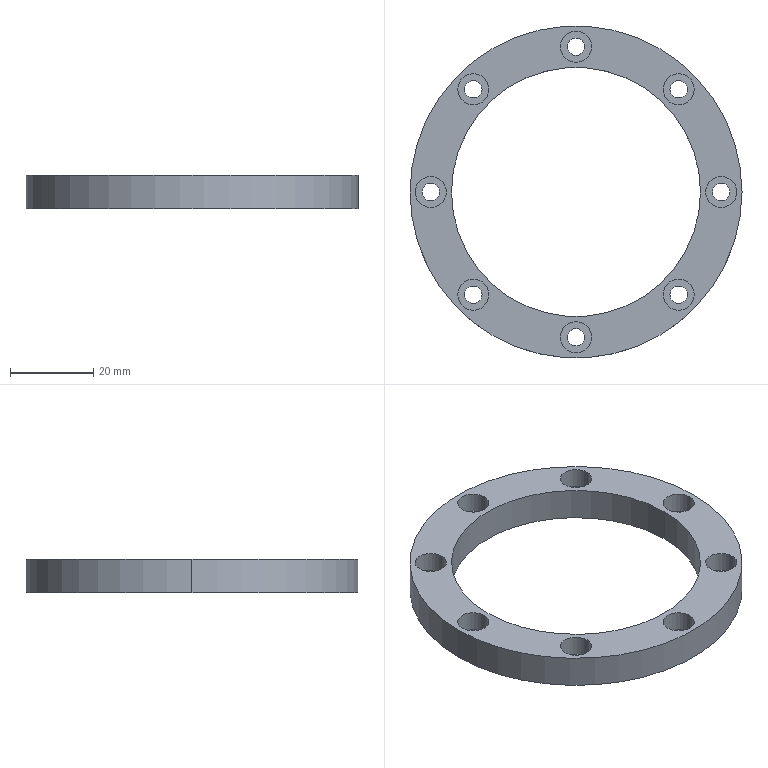Part | SolidWorks | features CirPattern 1, Extrusion 1, HoleWzd 1 | 1 solid | 46 faces | box 80 x 80 x 8 mm | volume 15493 mm3 | cylinder 36 | plane 10 | commonest cylinder face diameters 4.2 x16 7.5 x16 60 x2 80 x2
STEP:
#1=CARTESIAN_POINT('',(20.999,24.749,-1.));
#2=VERTEX_POINT('',#1);
#3=CARTESIAN_POINT('',(28.499,24.749,-1.));
#4=VERTEX_POINT('',#3);
#5=CARTESIAN_POINT('',(24.749,24.749,-1.));
#6=DIRECTION('',(0.,0.,1.));
#7=DIRECTION('',(1.,0.,0.));
#8=AXIS2_PLACEMENT_3D('',#5,#6,#7);
#9=CIRCLE('',#8,3.75);
#10=EDGE_CURVE('',#2,#4,#9,.T.);
#11=ORIENTED_EDGE('',*,*,#10,.F.);
#12=CARTESIAN_POINT('',(20.999,24.749,4.));
#13=VERTEX_POINT('',#12);
#14=CARTESIAN_POINT('',(20.999,24.749,4.));
#15=DIRECTION('',(0.,0.,1.));
#16=VECTOR('',#15,1000.);
#17=LINE('',#14,#16);
#18=EDGE_CURVE('',#2,#13,#17,.T.);
#19=ORIENTED_EDGE('',*,*,#18,.T.);
#20=CARTESIAN_POINT('',(28.499,24.749,4.));
#21=VERTEX_POINT('',#20);
#22=CARTESIAN_POINT('',(24.749,24.749,4.));
#23=DIRECTION('',(0.,0.,1.));
#24=DIRECTION('',(1.,0.,0.));
#25=AXIS2_PLACEMENT_3D('',#22,#23,#24);
#26=CIRCLE('',#25,3.75);
#27=EDGE_CURVE('',#13,#21,#26,.T.);
#28=ORIENTED_EDGE('',*,*,#27,.T.);
#29=CARTESIAN_POINT('',(28.499,24.749,4.));
#30=DIRECTION('',(0.,0.,1.));
#31=VECTOR('',#30,1000.);
#32=LINE('',#29,#31);
#33=EDGE_CURVE('',#4,#21,#32,.T.);
#34=ORIENTED_EDGE('',*,*,#33,.F.);
#35=EDGE_LOOP('',(#11,#19,#28,#34));
#36=FACE_OUTER_BOUND('',#35,.T.);
#37=CARTESIAN_POINT('',(24.749,24.749,4.));
#38=DIRECTION('',(0.,0.,1.));
#39=DIRECTION('',(1.,0.,0.));
#40=AXIS2_PLACEMENT_3D('',#37,#38,#39);
#41=CYLINDRICAL_SURFACE('',#40,3.75);
#42=ADVANCED_FACE('',(#36),#41,.F.);
#43=CARTESIAN_POINT('',(22.649,24.749,-4.));
#44=VERTEX_POINT('',#43);
#45=CARTESIAN_POINT('',(26.849,24.749,-4.));
#46=VERTEX_POINT('',#45);
#47=CARTESIAN_POINT('',(24.749,24.749,-4.));
#48=DIRECTION('',(0.,0.,1.));
#49=DIRECTION('',(1.,0.,0.));
#50=AXIS2_PLACEMENT_3D('',#47,#48,#49);
#51=CIRCLE('',#50,2.1);
#52=EDGE_CURVE('',#44,#46,#51,.T.);
#53=ORIENTED_EDGE('',*,*,#52,.F.);
#54=CARTESIAN_POINT('',(22.649,24.749,-1.));
#55=VERTEX_POINT('',#54);
#56=CARTESIAN_POINT('',(22.649,24.749,4.));
#57=DIRECTION('',(0.,0.,1.));
#58=VECTOR('',#57,1000.);
#59=LINE('',#56,#58);
#60=EDGE_CURVE('',#44,#55,#59,.T.);
#61=ORIENTED_EDGE('',*,*,#60,.T.);
#62=CARTESIAN_POINT('',(26.849,24.749,-1.));
#63=VERTEX_POINT('',#62);
#64=CARTESIAN_POINT('',(24.749,24.749,-1.));
#65=DIRECTION('',(0.,0.,1.));
#66=DIRECTION('',(1.,0.,0.));
#67=AXIS2_PLACEMENT_3D('',#64,#65,#66);
#68=CIRCLE('',#67,2.1);
#69=EDGE_CURVE('',#55,#63,#68,.T.);
#70=ORIENTED_EDGE('',*,*,#69,.T.);
#71=CARTESIAN_POINT('',(26.849,24.749,4.));
#72=DIRECTION('',(0.,0.,1.));
#73=VECTOR('',#72,1000.);
#74=LINE('',#71,#73);
#75=EDGE_CURVE('',#46,#63,#74,.T.);
#76=ORIENTED_EDGE('',*,*,#75,.F.);
#77=EDGE_LOOP('',(#53,#61,#70,#76));
#78=FACE_OUTER_BOUND('',#77,.T.);
#79=CARTESIAN_POINT('',(24.749,24.749,4.));
#80=DIRECTION('',(0.,0.,1.));
#81=DIRECTION('',(1.,0.,0.));
#82=AXIS2_PLACEMENT_3D('',#79,#80,#81);
#83=CYLINDRICAL_SURFACE('',#82,2.1);
#84=ADVANCED_FACE('',(#78),#83,.F.);
#85=CARTESIAN_POINT('',(-3.75,35.,-1.));
#86=VERTEX_POINT('',#85);
#87=CARTESIAN_POINT('',(3.75,35.,-1.));
#88=VERTEX_POINT('',#87);
#89=CARTESIAN_POINT('',(0.,35.,-1.));
#90=DIRECTION('',(0.,0.,1.));
#91=DIRECTION('',(1.,0.,0.));
#92=AXIS2_PLACEMENT_3D('',#89,#90,#91);
#93=CIRCLE('',#92,3.75);
#94=EDGE_CURVE('',#86,#88,#93,.T.);
#95=ORIENTED_EDGE('',*,*,#94,.F.);
#96=CARTESIAN_POINT('',(-3.75,35.,4.));
#97=VERTEX_POINT('',#96);
#98=CARTESIAN_POINT('',(-3.75,35.,4.));
#99=DIRECTION('',(0.,0.,1.));
#100=VECTOR('',#99,1000.);
#101=LINE('',#98,#100);
#102=EDGE_CURVE('',#86,#97,#101,.T.);
#103=ORIENTED_EDGE('',*,*,#102,.T.);
#104=CARTESIAN_POINT('',(3.75,35.,4.));
#105=VERTEX_POINT('',#104);
#106=CARTESIAN_POINT('',(0.,35.,4.));
#107=DIRECTION('',(0.,0.,1.));
#108=DIRECTION('',(1.,0.,0.));
#109=AXIS2_PLACEMENT_3D('',#106,#107,#108);
#110=CIRCLE('',#109,3.75);
#111=EDGE_CURVE('',#97,#105,#110,.T.);
#112=ORIENTED_EDGE('',*,*,#111,.T.);
#113=CARTESIAN_POINT('',(3.75,35.,4.));
#114=DIRECTION('',(0.,0.,1.));
#115=VECTOR('',#114,1000.);
#116=LINE('',#113,#115);
#117=EDGE_CURVE('',#88,#105,#116,.T.);
#118=ORIENTED_EDGE('',*,*,#117,.F.);
#119=EDGE_LOOP('',(#95,#103,#112,#118));
#120=FACE_OUTER_BOUND('',#119,.T.);
#121=CARTESIAN_POINT('',(0.,35.,4.));
#122=DIRECTION('',(0.,0.,1.));
#123=DIRECTION('',(1.,0.,0.));
#124=AXIS2_PLACEMENT_3D('',#121,#122,#123);
#125=CYLINDRICAL_SURFACE('',#124,3.75);
#126=ADVANCED_FACE('',(#120),#125,.F.);
#127=CARTESIAN_POINT('',(-2.1,35.,-4.));
#128=VERTEX_POINT('',#127);
#129=CARTESIAN_POINT('',(2.1,35.,-4.));
#130=VERTEX_POINT('',#129);
#131=CARTESIAN_POINT('',(0.,35.,-4.));
#132=DIRECTION('',(0.,0.,1.));
#133=DIRECTION('',(1.,0.,0.));
#134=AXIS2_PLACEMENT_3D('',#131,#132,#133);
#135=CIRCLE('',#134,2.1);
#136=EDGE_CURVE('',#128,#130,#135,.T.);
#137=ORIENTED_EDGE('',*,*,#136,.F.);
#138=CARTESIAN_POINT('',(-2.1,35.,-1.));
#139=VERTEX_POINT('',#138);
#140=CARTESIAN_POINT('',(-2.1,35.,4.));
#141=DIRECTION('',(0.,0.,1.));
#142=VECTOR('',#141,1000.);
#143=LINE('',#140,#142);
#144=EDGE_CURVE('',#128,#139,#143,.T.);
#145=ORIENTED_EDGE('',*,*,#144,.T.);
#146=CARTESIAN_POINT('',(2.1,35.,-1.));
#147=VERTEX_POINT('',#146);
#148=CARTESIAN_POINT('',(0.,35.,-1.));
#149=DIRECTION('',(0.,0.,1.));
#150=DIRECTION('',(1.,0.,0.));
#151=AXIS2_PLACEMENT_3D('',#148,#149,#150);
#152=CIRCLE('',#151,2.1);
#153=EDGE_CURVE('',#139,#147,#152,.T.);
#154=ORIENTED_EDGE('',*,*,#153,.T.);
#155=CARTESIAN_POINT('',(2.1,35.,4.));
#156=DIRECTION('',(0.,0.,1.));
#157=VECTOR('',#156,1000.);
#158=LINE('',#155,#157);
#159=EDGE_CURVE('',#130,#147,#158,.T.);
#160=ORIENTED_EDGE('',*,*,#159,.F.);
#161=EDGE_LOOP('',(#137,#145,#154,#160));
#162=FACE_OUTER_BOUND('',#161,.T.);
#163=CARTESIAN_POINT('',(0.,35.,4.));
#164=DIRECTION('',(0.,0.,1.));
#165=DIRECTION('',(1.,0.,0.));
#166=AXIS2_PLACEMENT_3D('',#163,#164,#165);
#167=CYLINDRICAL_SURFACE('',#166,2.1);
#168=ADVANCED_FACE('',(#162),#167,.F.);
#169=CARTESIAN_POINT('',(-28.499,24.749,-1.));
#170=VERTEX_POINT('',#169);
#171=CARTESIAN_POINT('',(-20.999,24.749,-1.));
#172=VERTEX_POINT('',#171);
#173=CARTESIAN_POINT('',(-24.749,24.749,-1.));
#174=DIRECTION('',(0.,0.,1.));
#175=DIRECTION('',(1.,0.,0.));
#176=AXIS2_PLACEMENT_3D('',#173,#174,#175);
#177=CIRCLE('',#176,3.75);
#178=EDGE_CURVE('',#170,#172,#177,.T.);
#179=ORIENTED_EDGE('',*,*,#178,.F.);
#180=CARTESIAN_POINT('',(-28.499,24.749,4.));
#181=VERTEX_POINT('',#180);
#182=CARTESIAN_POINT('',(-28.499,24.749,4.));
#183=DIRECTION('',(0.,0.,1.));
#184=VECTOR('',#183,1000.);
#185=LINE('',#182,#184);
#186=EDGE_CURVE('',#170,#181,#185,.T.);
#187=ORIENTED_EDGE('',*,*,#186,.T.);
#188=CARTESIAN_POINT('',(-20.999,24.749,4.));
#189=VERTEX_POINT('',#188);
#190=CARTESIAN_POINT('',(-24.749,24.749,4.));
#191=DIRECTION('',(0.,0.,1.));
#192=DIRECTION('',(1.,0.,0.));
#193=AXIS2_PLACEMENT_3D('',#190,#191,#192);
#194=CIRCLE('',#193,3.75);
#195=EDGE_CURVE('',#181,#189,#194,.T.);
#196=ORIENTED_EDGE('',*,*,#195,.T.);
#197=CARTESIAN_POINT('',(-20.999,24.749,4.));
#198=DIRECTION('',(0.,0.,1.));
#199=VECTOR('',#198,1000.);
#200=LINE('',#197,#199);
#201=EDGE_CURVE('',#172,#189,#200,.T.);
#202=ORIENTED_EDGE('',*,*,#201,.F.);
#203=EDGE_LOOP('',(#179,#187,#196,#202));
#204=FACE_OUTER_BOUND('',#203,.T.);
#205=CARTESIAN_POINT('',(-24.749,24.749,4.));
#206=DIRECTION('',(0.,0.,1.));
#207=DIRECTION('',(1.,0.,0.));
#208=AXIS2_PLACEMENT_3D('',#205,#206,#207);
#209=CYLINDRICAL_SURFACE('',#208,3.75);
#210=ADVANCED_FACE('',(#204),#209,.F.);
#211=CARTESIAN_POINT('',(-26.849,24.749,-4.));
#212=VERTEX_POINT('',#211);
#213=CARTESIAN_POINT('',(-22.649,24.749,-4.));
#214=VERTEX_POINT('',#213);
#215=CARTESIAN_POINT('',(-24.749,24.749,-4.));
#216=DIRECTION('',(0.,0.,1.));
#217=DIRECTION('',(1.,0.,0.));
#218=AXIS2_PLACEMENT_3D('',#215,#216,#217);
#219=CIRCLE('',#218,2.1);
#220=EDGE_CURVE('',#212,#214,#219,.T.);
#221=ORIENTED_EDGE('',*,*,#220,.F.);
#222=CARTESIAN_POINT('',(-26.849,24.749,-1.));
#223=VERTEX_POINT('',#222);
#224=CARTESIAN_POINT('',(-26.849,24.749,4.));
#225=DIRECTION('',(0.,0.,1.));
#226=VECTOR('',#225,1000.);
#227=LINE('',#224,#226);
#228=EDGE_CURVE('',#212,#223,#227,.T.);
#229=ORIENTED_EDGE('',*,*,#228,.T.);
#230=CARTESIAN_POINT('',(-22.649,24.749,-1.));
#231=VERTEX_POINT('',#230);
#232=CARTESIAN_POINT('',(-24.749,24.749,-1.));
#233=DIRECTION('',(0.,0.,1.));
#234=DIRECTION('',(1.,0.,0.));
#235=AXIS2_PLACEMENT_3D('',#232,#233,#234);
#236=CIRCLE('',#235,2.1);
#237=EDGE_CURVE('',#223,#231,#236,.T.);
#238=ORIENTED_EDGE('',*,*,#237,.T.);
#239=CARTESIAN_POINT('',(-22.649,24.749,4.));
#240=DIRECTION('',(0.,0.,1.));
#241=VECTOR('',#240,1000.);
#242=LINE('',#239,#241);
#243=EDGE_CURVE('',#214,#231,#242,.T.);
#244=ORIENTED_EDGE('',*,*,#243,.F.);
#245=EDGE_LOOP('',(#221,#229,#238,#244));
#246=FACE_OUTER_BOUND('',#245,.T.);
#247=CARTESIAN_POINT('',(-24.749,24.749,4.));
#248=DIRECTION('',(0.,0.,1.));
#249=DIRECTION('',(1.,0.,0.));
#250=AXIS2_PLACEMENT_3D('',#247,#248,#249);
#251=CYLINDRICAL_SURFACE('',#250,2.1);
#252=ADVANCED_FACE('',(#246),#251,.F.);
#253=CARTESIAN_POINT('',(-38.75,0.,-1.));
#254=VERTEX_POINT('',#253);
#255=CARTESIAN_POINT('',(-31.25,0.,-1.));
#256=VERTEX_POINT('',#255);
#257=CARTESIAN_POINT('',(-35.,0.,-1.));
#258=DIRECTION('',(0.,0.,1.));
#259=DIRECTION('',(1.,0.,0.));
#260=AXIS2_PLACEMENT_3D('',#257,#258,#259);
#261=CIRCLE('',#260,3.75);
#262=EDGE_CURVE('',#254,#256,#261,.T.);
#263=ORIENTED_EDGE('',*,*,#262,.F.);
#264=CARTESIAN_POINT('',(-38.75,0.,4.));
#265=VERTEX_POINT('',#264);
#266=CARTESIAN_POINT('',(-38.75,0.,4.));
#267=DIRECTION('',(0.,0.,1.));
#268=VECTOR('',#267,1000.);
#269=LINE('',#266,#268);
#270=EDGE_CURVE('',#254,#265,#269,.T.);
#271=ORIENTED_EDGE('',*,*,#270,.T.);
#272=CARTESIAN_POINT('',(-31.25,0.,4.));
#273=VERTEX_POINT('',#272);
#274=CARTESIAN_POINT('',(-35.,0.,4.));
#275=DIRECTION('',(0.,0.,1.));
#276=DIRECTION('',(1.,0.,0.));
#277=AXIS2_PLACEMENT_3D('',#274,#275,#276);
#278=CIRCLE('',#277,3.75);
#279=EDGE_CURVE('',#265,#273,#278,.T.);
#280=ORIENTED_EDGE('',*,*,#279,.T.);
#281=CARTESIAN_POINT('',(-31.25,0.,4.));
#282=DIRECTION('',(0.,0.,1.));
#283=VECTOR('',#282,1000.);
#284=LINE('',#281,#283);
#285=EDGE_CURVE('',#256,#273,#284,.T.);
#286=ORIENTED_EDGE('',*,*,#285,.F.);
#287=EDGE_LOOP('',(#263,#271,#280,#286));
#288=FACE_OUTER_BOUND('',#287,.T.);
#289=CARTESIAN_POINT('',(-35.,0.,4.));
#290=DIRECTION('',(0.,0.,1.));
#291=DIRECTION('',(1.,0.,0.));
#292=AXIS2_PLACEMENT_3D('',#289,#290,#291);
#293=CYLINDRICAL_SURFACE('',#292,3.75);
#294=ADVANCED_FACE('',(#288),#293,.F.);
#295=CARTESIAN_POINT('',(-37.1,0.,-4.));
#296=VERTEX_POINT('',#295);
#297=CARTESIAN_POINT('',(-32.9,0.,-4.));
#298=VERTEX_POINT('',#297);
#299=CARTESIAN_POINT('',(-35.,0.,-4.));
#300=DIRECTION('',(0.,0.,1.));
#301=DIRECTION('',(1.,0.,0.));
#302=AXIS2_PLACEMENT_3D('',#299,#300,#301);
#303=CIRCLE('',#302,2.1);
#304=EDGE_CURVE('',#296,#298,#303,.T.);
#305=ORIENTED_EDGE('',*,*,#304,.F.);
#306=CARTESIAN_POINT('',(-37.1,0.,-1.));
#307=VERTEX_POINT('',#306);
#308=CARTESIAN_POINT('',(-37.1,0.,4.));
#309=DIRECTION('',(0.,0.,1.));
#310=VECTOR('',#309,1000.);
#311=LINE('',#308,#310);
#312=EDGE_CURVE('',#296,#307,#311,.T.);
#313=ORIENTED_EDGE('',*,*,#312,.T.);
#314=CARTESIAN_POINT('',(-32.9,0.,-1.));
#315=VERTEX_POINT('',#314);
#316=CARTESIAN_POINT('',(-35.,0.,-1.));
#317=DIRECTION('',(0.,0.,1.));
#318=DIRECTION('',(1.,0.,0.));
#319=AXIS2_PLACEMENT_3D('',#316,#317,#318);
#320=CIRCLE('',#319,2.1);
#321=EDGE_CURVE('',#307,#315,#320,.T.);
#322=ORIENTED_EDGE('',*,*,#321,.T.);
#323=CARTESIAN_POINT('',(-32.9,0.,4.));
#324=DIRECTION('',(0.,0.,1.));
#325=VECTOR('',#324,1000.);
#326=LINE('',#323,#325);
#327=EDGE_CURVE('',#298,#315,#326,.T.);
#328=ORIENTED_EDGE('',*,*,#327,.F.);
#329=EDGE_LOOP('',(#305,#313,#322,#328));
#330=FACE_OUTER_BOUND('',#329,.T.);
#331=CARTESIAN_POINT('',(-35.,0.,4.));
#332=DIRECTION('',(0.,0.,1.));
#333=DIRECTION('',(1.,0.,0.));
#334=AXIS2_PLACEMENT_3D('',#331,#332,#333);
#335=CYLINDRICAL_SURFACE('',#334,2.1);
#336=ADVANCED_FACE('',(#330),#335,.F.);
#337=CARTESIAN_POINT('',(-28.499,-24.749,-1.));
#338=VERTEX_POINT('',#337);
#339=CARTESIAN_POINT('',(-20.999,-24.749,-1.));
#340=VERTEX_POINT('',#339);
#341=CARTESIAN_POINT('',(-24.749,-24.749,-1.));
#342=DIRECTION('',(0.,0.,1.));
#343=DIRECTION('',(1.,0.,0.));
#344=AXIS2_PLACEMENT_3D('',#341,#342,#343);
#345=CIRCLE('',#344,3.75);
#346=EDGE_CURVE('',#338,#340,#345,.T.);
#347=ORIENTED_EDGE('',*,*,#346,.F.);
#348=CARTESIAN_POINT('',(-28.499,-24.749,4.));
#349=VERTEX_POINT('',#348);
#350=CARTESIAN_POINT('',(-28.499,-24.749,4.));
#351=DIRECTION('',(0.,0.,1.));
#352=VECTOR('',#351,1000.);
#353=LINE('',#350,#352);
#354=EDGE_CURVE('',#338,#349,#353,.T.);
#355=ORIENTED_EDGE('',*,*,#354,.T.);
#356=CARTESIAN_POINT('',(-20.999,-24.749,4.));
#357=VERTEX_POINT('',#356);
#358=CARTESIAN_POINT('',(-24.749,-24.749,4.));
#359=DIRECTION('',(0.,0.,1.));
#360=DIRECTION('',(1.,0.,0.));
#361=AXIS2_PLACEMENT_3D('',#358,#359,#360);
#362=CIRCLE('',#361,3.75);
#363=EDGE_CURVE('',#349,#357,#362,.T.);
#364=ORIENTED_EDGE('',*,*,#363,.T.);
#365=CARTESIAN_POINT('',(-20.999,-24.749,4.));
#366=DIRECTION('',(0.,0.,1.));
#367=VECTOR('',#366,1000.);
#368=LINE('',#365,#367);
#369=EDGE_CURVE('',#340,#357,#368,.T.);
#370=ORIENTED_EDGE('',*,*,#369,.F.);
#371=EDGE_LOOP('',(#347,#355,#364,#370));
#372=FACE_OUTER_BOUND('',#371,.T.);
#373=CARTESIAN_POINT('',(-24.749,-24.749,4.));
#374=DIRECTION('',(0.,0.,1.));
#375=DIRECTION('',(1.,0.,0.));
#376=AXIS2_PLACEMENT_3D('',#373,#374,#375);
#377=CYLINDRICAL_SURFACE('',#376,3.75);
#378=ADVANCED_FACE('',(#372),#377,.F.);
#379=CARTESIAN_POINT('',(-26.849,-24.749,-4.));
#380=VERTEX_POINT('',#379);
#381=CARTESIAN_POINT('',(-22.649,-24.749,-4.));
#382=VERTEX_POINT('',#381);
#383=CARTESIAN_POINT('',(-24.749,-24.749,-4.));
#384=DIRECTION('',(0.,0.,1.));
#385=DIRECTION('',(1.,0.,0.));
#386=AXIS2_PLACEMENT_3D('',#383,#384,#385);
#387=CIRCLE('',#386,2.1);
#388=EDGE_CURVE('',#380,#382,#387,.T.);
#389=ORIENTED_EDGE('',*,*,#388,.F.);
#390=CARTESIAN_POINT('',(-26.849,-24.749,-1.));
#391=VERTEX_POINT('',#390);
#392=CARTESIAN_POINT('',(-26.849,-24.749,4.));
#393=DIRECTION('',(0.,0.,1.));
#394=VECTOR('',#393,1000.);
#395=LINE('',#392,#394);
#396=EDGE_CURVE('',#380,#391,#395,.T.);
#397=ORIENTED_EDGE('',*,*,#396,.T.);
#398=CARTESIAN_POINT('',(-22.649,-24.749,-1.));
#399=VERTEX_POINT('',#398);
#400=CARTESIAN_POINT('',(-24.749,-24.749,-1.));
#401=DIRECTION('',(0.,0.,1.));
#402=DIRECTION('',(1.,0.,0.));
#403=AXIS2_PLACEMENT_3D('',#400,#401,#402);
#404=CIRCLE('',#403,2.1);
#405=EDGE_CURVE('',#391,#399,#404,.T.);
#406=ORIENTED_EDGE('',*,*,#405,.T.);
#407=CARTESIAN_POINT('',(-22.649,-24.749,4.));
#408=DIRECTION('',(0.,0.,1.));
#409=VECTOR('',#408,1000.);
#410=LINE('',#407,#409);
#411=EDGE_CURVE('',#382,#399,#410,.T.);
#412=ORIENTED_EDGE('',*,*,#411,.F.);
#413=EDGE_LOOP('',(#389,#397,#406,#412));
#414=FACE_OUTER_BOUND('',#413,.T.);
#415=CARTESIAN_POINT('',(-24.749,-24.749,4.));
#416=DIRECTION('',(0.,0.,1.));
#417=DIRECTION('',(1.,0.,0.));
#418=AXIS2_PLACEMENT_3D('',#415,#416,#417);
#419=CYLINDRICAL_SURFACE('',#418,2.1);
#420=ADVANCED_FACE('',(#414),#419,.F.);
#421=CARTESIAN_POINT('',(-3.75,-35.,-1.));
#422=VERTEX_POINT('',#421);
#423=CARTESIAN_POINT('',(3.75,-35.,-1.));
#424=VERTEX_POINT('',#423);
#425=CARTESIAN_POINT('',(0.,-35.,-1.));
#426=DIRECTION('',(0.,0.,1.));
#427=DIRECTION('',(1.,0.,0.));
#428=AXIS2_PLACEMENT_3D('',#425,#426,#427);
#429=CIRCLE('',#428,3.75);
#430=EDGE_CURVE('',#422,#424,#429,.T.);
#431=ORIENTED_EDGE('',*,*,#430,.F.);
#432=CARTESIAN_POINT('',(-3.75,-35.,4.));
#433=VERTEX_POINT('',#432);
#434=CARTESIAN_POINT('',(-3.75,-35.,4.));
#435=DIRECTION('',(0.,0.,1.));
#436=VECTOR('',#435,1000.);
#437=LINE('',#434,#436);
#438=EDGE_CURVE('',#422,#433,#437,.T.);
#439=ORIENTED_EDGE('',*,*,#438,.T.);
#440=CARTESIAN_POINT('',(3.75,-35.,4.));
#441=VERTEX_POINT('',#440);
#442=CARTESIAN_POINT('',(0.,-35.,4.));
#443=DIRECTION('',(0.,0.,1.));
#444=DIRECTION('',(1.,0.,0.));
#445=AXIS2_PLACEMENT_3D('',#442,#443,#444);
#446=CIRCLE('',#445,3.75);
#447=EDGE_CURVE('',#433,#441,#446,.T.);
#448=ORIENTED_EDGE('',*,*,#447,.T.);
#449=CARTESIAN_POINT('',(3.75,-35.,4.));
#450=DIRECTION('',(0.,0.,1.));
#451=VECTOR('',#450,1000.);
#452=LINE('',#449,#451);
#453=EDGE_CURVE('',#424,#441,#452,.T.);
#454=ORIENTED_EDGE('',*,*,#453,.F.);
#455=EDGE_LOOP('',(#431,#439,#448,#454));
#456=FACE_OUTER_BOUND('',#455,.T.);
#457=CARTESIAN_POINT('',(0.,-35.,4.));
#458=DIRECTION('',(0.,0.,1.));
#459=DIRECTION('',(1.,0.,0.));
#460=AXIS2_PLACEMENT_3D('',#457,#458,#459);
#461=CYLINDRICAL_SURFACE('',#460,3.75);
#462=ADVANCED_FACE('',(#456),#461,.F.);
#463=CARTESIAN_POINT('',(-2.1,-35.,-4.));
#464=VERTEX_POINT('',#463);
#465=CARTESIAN_POINT('',(2.1,-35.,-4.));
#466=VERTEX_POINT('',#465);
#467=CARTESIAN_POINT('',(0.,-35.,-4.));
#468=DIRECTION('',(0.,0.,1.));
#469=DIRECTION('',(1.,0.,0.));
#470=AXIS2_PLACEMENT_3D('',#467,#468,#469);
#471=CIRCLE('',#470,2.1);
#472=EDGE_CURVE('',#464,#466,#471,.T.);
#473=ORIENTED_EDGE('',*,*,#472,.F.);
#474=CARTESIAN_POINT('',(-2.1,-35.,-1.));
#475=VERTEX_POINT('',#474);
#476=CARTESIAN_POINT('',(-2.1,-35.,4.));
#477=DIRECTION('',(0.,0.,1.));
#478=VECTOR('',#477,1000.);
#479=LINE('',#476,#478);
#480=EDGE_CURVE('',#464,#475,#479,.T.);
#481=ORIENTED_EDGE('',*,*,#480,.T.);
#482=CARTESIAN_POINT('',(2.1,-35.,-1.));
#483=VERTEX_POINT('',#482);
#484=CARTESIAN_POINT('',(0.,-35.,-1.));
#485=DIRECTION('',(0.,0.,1.));
#486=DIRECTION('',(1.,0.,0.));
#487=AXIS2_PLACEMENT_3D('',#484,#485,#486);
#488=CIRCLE('',#487,2.1);
#489=EDGE_CURVE('',#475,#483,#488,.T.);
#490=ORIENTED_EDGE('',*,*,#489,.T.);
#491=CARTESIAN_POINT('',(2.1,-35.,4.));
#492=DIRECTION('',(0.,0.,1.));
#493=VECTOR('',#492,1000.);
#494=LINE('',#491,#493);
#495=EDGE_CURVE('',#466,#483,#494,.T.);
#496=ORIENTED_EDGE('',*,*,#495,.F.);
#497=EDGE_LOOP('',(#473,#481,#490,#496));
#498=FACE_OUTER_BOUND('',#497,.T.);
#499=CARTESIAN_POINT('',(0.,-35.,4.));
#500=DIRECTION('',(0.,0.,1.));
#501=DIRECTION('',(1.,0.,0.));
#502=AXIS2_PLACEMENT_3D('',#499,#500,#501);
#503=CYLINDRICAL_SURFACE('',#502,2.1);
#504=ADVANCED_FACE('',(#498),#503,.F.);
#505=CARTESIAN_POINT('',(20.999,-24.749,-1.));
#506=VERTEX_POINT('',#505);
#507=CARTESIAN_POINT('',(28.499,-24.749,-1.));
#508=VERTEX_POINT('',#507);
#509=CARTESIAN_POINT('',(24.749,-24.749,-1.));
#510=DIRECTION('',(0.,0.,1.));
#511=DIRECTION('',(1.,0.,0.));
#512=AXIS2_PLACEMENT_3D('',#509,#510,#511);
#513=CIRCLE('',#512,3.75);
#514=EDGE_CURVE('',#506,#508,#513,.T.);
#515=ORIENTED_EDGE('',*,*,#514,.F.);
#516=CARTESIAN_POINT('',(20.999,-24.749,4.));
#517=VERTEX_POINT('',#516);
#518=CARTESIAN_POINT('',(20.999,-24.749,4.));
#519=DIRECTION('',(0.,0.,1.));
#520=VECTOR('',#519,1000.);
#521=LINE('',#518,#520);
#522=EDGE_CURVE('',#506,#517,#521,.T.);
#523=ORIENTED_EDGE('',*,*,#522,.T.);
#524=CARTESIAN_POINT('',(28.499,-24.749,4.));
#525=VERTEX_POINT('',#524);
#526=CARTESIAN_POINT('',(24.749,-24.749,4.));
#527=DIRECTION('',(0.,0.,1.));
#528=DIRECTION('',(1.,0.,0.));
#529=AXIS2_PLACEMENT_3D('',#526,#527,#528);
#530=CIRCLE('',#529,3.75);
#531=EDGE_CURVE('',#517,#525,#530,.T.);
#532=ORIENTED_EDGE('',*,*,#531,.T.);
#533=CARTESIAN_POINT('',(28.499,-24.749,4.));
#534=DIRECTION('',(0.,0.,1.));
#535=VECTOR('',#534,1000.);
#536=LINE('',#533,#535);
#537=EDGE_CURVE('',#508,#525,#536,.T.);
#538=ORIENTED_EDGE('',*,*,#537,.F.);
#539=EDGE_LOOP('',(#515,#523,#532,#538));
#540=FACE_OUTER_BOUND('',#539,.T.);
#541=CARTESIAN_POINT('',(24.749,-24.749,4.));
#542=DIRECTION('',(0.,0.,1.));
#543=DIRECTION('',(1.,0.,0.));
#544=AXIS2_PLACEMENT_3D('',#541,#542,#543);
#545=CYLINDRICAL_SURFACE('',#544,3.75);
#546=ADVANCED_FACE('',(#540),#545,.F.);
#547=CARTESIAN_POINT('',(22.649,-24.749,-4.));
#548=VERTEX_POINT('',#547);
#549=CARTESIAN_POINT('',(26.849,-24.749,-4.));
#550=VERTEX_POINT('',#549);
#551=CARTESIAN_POINT('',(24.749,-24.749,-4.));
#552=DIRECTION('',(0.,0.,1.));
#553=DIRECTION('',(1.,0.,0.));
#554=AXIS2_PLACEMENT_3D('',#551,#552,#553);
#555=CIRCLE('',#554,2.1);
#556=EDGE_CURVE('',#548,#550,#555,.T.);
#557=ORIENTED_EDGE('',*,*,#556,.F.);
#558=CARTESIAN_POINT('',(22.649,-24.749,-1.));
#559=VERTEX_POINT('',#558);
#560=CARTESIAN_POINT('',(22.649,-24.749,4.));
#561=DIRECTION('',(0.,0.,1.));
#562=VECTOR('',#561,1000.);
#563=LINE('',#560,#562);
#564=EDGE_CURVE('',#548,#559,#563,.T.);
#565=ORIENTED_EDGE('',*,*,#564,.T.);
#566=CARTESIAN_POINT('',(26.849,-24.749,-1.));
#567=VERTEX_POINT('',#566);
#568=CARTESIAN_POINT('',(24.749,-24.749,-1.));
#569=DIRECTION('',(0.,0.,1.));
#570=DIRECTION('',(1.,0.,0.));
#571=AXIS2_PLACEMENT_3D('',#568,#569,#570);
#572=CIRCLE('',#571,2.1);
#573=EDGE_CURVE('',#559,#567,#572,.T.);
#574=ORIENTED_EDGE('',*,*,#573,.T.);
#575=CARTESIAN_POINT('',(26.849,-24.749,4.));
#576=DIRECTION('',(0.,0.,1.));
#577=VECTOR('',#576,1000.);
#578=LINE('',#575,#577);
#579=EDGE_CURVE('',#550,#567,#578,.T.);
#580=ORIENTED_EDGE('',*,*,#579,.F.);
#581=EDGE_LOOP('',(#557,#565,#574,#580));
#582=FACE_OUTER_BOUND('',#581,.T.);
#583=CARTESIAN_POINT('',(24.749,-24.749,4.));
#584=DIRECTION('',(0.,0.,1.));
#585=DIRECTION('',(1.,0.,0.));
#586=AXIS2_PLACEMENT_3D('',#583,#584,#585);
#587=CYLINDRICAL_SURFACE('',#586,2.1);
#588=ADVANCED_FACE('',(#582),#587,.F.);
#589=CARTESIAN_POINT('',(31.25,0.,-1.));
#590=VERTEX_POINT('',#589);
#591=CARTESIAN_POINT('',(38.75,0.,-1.));
#592=VERTEX_POINT('',#591);
#593=CARTESIAN_POINT('',(35.,0.,-1.));
#594=DIRECTION('',(0.,0.,1.));
#595=DIRECTION('',(1.,0.,0.));
#596=AXIS2_PLACEMENT_3D('',#593,#594,#595);
#597=CIRCLE('',#596,3.75);
#598=EDGE_CURVE('',#590,#592,#597,.T.);
#599=ORIENTED_EDGE('',*,*,#598,.F.);
#600=CARTESIAN_POINT('',(31.25,0.,4.));
#601=VERTEX_POINT('',#600);
#602=CARTESIAN_POINT('',(31.25,0.,4.));
#603=DIRECTION('',(0.,0.,1.));
#604=VECTOR('',#603,1000.);
#605=LINE('',#602,#604);
#606=EDGE_CURVE('',#590,#601,#605,.T.);
#607=ORIENTED_EDGE('',*,*,#606,.T.);
#608=CARTESIAN_POINT('',(38.75,0.,4.));
#609=VERTEX_POINT('',#608);
#610=CARTESIAN_POINT('',(35.,0.,4.));
#611=DIRECTION('',(0.,0.,1.));
#612=DIRECTION('',(1.,0.,0.));
#613=AXIS2_PLACEMENT_3D('',#610,#611,#612);
#614=CIRCLE('',#613,3.75);
#615=EDGE_CURVE('',#601,#609,#614,.T.);
#616=ORIENTED_EDGE('',*,*,#615,.T.);
#617=CARTESIAN_POINT('',(38.75,0.,4.));
#618=DIRECTION('',(0.,0.,1.));
#619=VECTOR('',#618,1000.);
#620=LINE('',#617,#619);
#621=EDGE_CURVE('',#592,#609,#620,.T.);
#622=ORIENTED_EDGE('',*,*,#621,.F.);
#623=EDGE_LOOP('',(#599,#607,#616,#622));
#624=FACE_OUTER_BOUND('',#623,.T.);
#625=CARTESIAN_POINT('',(35.,0.,4.));
#626=DIRECTION('',(0.,0.,1.));
#627=DIRECTION('',(1.,0.,0.));
#628=AXIS2_PLACEMENT_3D('',#625,#626,#627);
#629=CYLINDRICAL_SURFACE('',#628,3.75);
#630=ADVANCED_FACE('',(#624),#629,.F.);
#631=CARTESIAN_POINT('',(32.9,0.,-4.));
#632=VERTEX_POINT('',#631);
#633=CARTESIAN_POINT('',(37.1,0.,-4.));
#634=VERTEX_POINT('',#633);
#635=CARTESIAN_POINT('',(35.,0.,-4.));
#636=DIRECTION('',(0.,0.,1.));
#637=DIRECTION('',(1.,0.,0.));
#638=AXIS2_PLACEMENT_3D('',#635,#636,#637);
#639=CIRCLE('',#638,2.1);
#640=EDGE_CURVE('',#632,#634,#639,.T.);
#641=ORIENTED_EDGE('',*,*,#640,.F.);
#642=CARTESIAN_POINT('',(32.9,0.,-1.));
#643=VERTEX_POINT('',#642);
#644=CARTESIAN_POINT('',(32.9,0.,4.));
#645=DIRECTION('',(0.,0.,1.));
#646=VECTOR('',#645,1000.);
#647=LINE('',#644,#646);
#648=EDGE_CURVE('',#632,#643,#647,.T.);
#649=ORIENTED_EDGE('',*,*,#648,.T.);
#650=CARTESIAN_POINT('',(37.1,0.,-1.));
#651=VERTEX_POINT('',#650);
#652=CARTESIAN_POINT('',(35.,0.,-1.));
#653=DIRECTION('',(0.,0.,1.));
#654=DIRECTION('',(1.,0.,0.));
#655=AXIS2_PLACEMENT_3D('',#652,#653,#654);
#656=CIRCLE('',#655,2.1);
#657=EDGE_CURVE('',#643,#651,#656,.T.);
#658=ORIENTED_EDGE('',*,*,#657,.T.);
#659=CARTESIAN_POINT('',(37.1,0.,4.));
#660=DIRECTION('',(0.,0.,1.));
#661=VECTOR('',#660,1000.);
#662=LINE('',#659,#661);
#663=EDGE_CURVE('',#634,#651,#662,.T.);
#664=ORIENTED_EDGE('',*,*,#663,.F.);
#665=EDGE_LOOP('',(#641,#649,#658,#664));
#666=FACE_OUTER_BOUND('',#665,.T.);
#667=CARTESIAN_POINT('',(35.,0.,4.));
#668=DIRECTION('',(0.,0.,1.));
#669=DIRECTION('',(1.,0.,0.));
#670=AXIS2_PLACEMENT_3D('',#667,#668,#669);
#671=CYLINDRICAL_SURFACE('',#670,2.1);
#672=ADVANCED_FACE('',(#666),#671,.F.);
#673=CARTESIAN_POINT('',(-30.,0.,4.));
#674=VERTEX_POINT('',#673);
#675=CARTESIAN_POINT('',(30.,0.,4.));
#676=VERTEX_POINT('',#675);
#677=CARTESIAN_POINT('',(0.,0.,4.));
#678=DIRECTION('',(0.,0.,1.));
#679=DIRECTION('',(1.,0.,0.));
#680=AXIS2_PLACEMENT_3D('',#677,#678,#679);
#681=CIRCLE('',#680,30.);
#682=EDGE_CURVE('',#674,#676,#681,.T.);
#683=ORIENTED_EDGE('',*,*,#682,.T.);
#684=CARTESIAN_POINT('',(30.,0.,-4.));
#685=VERTEX_POINT('',#684);
#686=CARTESIAN_POINT('',(30.,0.,4.));
#687=DIRECTION('',(0.,0.,-1.));
#688=VECTOR('',#687,1000.);
#689=LINE('',#686,#688);
#690=EDGE_CURVE('',#676,#685,#689,.T.);
#691=ORIENTED_EDGE('',*,*,#690,.T.);
#692=CARTESIAN_POINT('',(-30.,0.,-4.));
#693=VERTEX_POINT('',#692);
#694=CARTESIAN_POINT('',(0.,0.,-4.));
#695=DIRECTION('',(0.,0.,1.));
#696=DIRECTION('',(1.,0.,0.));
#697=AXIS2_PLACEMENT_3D('',#694,#695,#696);
#698=CIRCLE('',#697,30.);
#699=EDGE_CURVE('',#693,#685,#698,.T.);
#700=ORIENTED_EDGE('',*,*,#699,.F.);
#701=CARTESIAN_POINT('',(-30.,0.,4.));
#702=DIRECTION('',(0.,0.,-1.));
#703=VECTOR('',#702,1000.);
#704=LINE('',#701,#703);
#705=EDGE_CURVE('',#674,#693,#704,.T.);
#706=ORIENTED_EDGE('',*,*,#705,.F.);
#707=EDGE_LOOP('',(#683,#691,#700,#706));
#708=FACE_OUTER_BOUND('',#707,.T.);
#709=CARTESIAN_POINT('',(0.,0.,4.));
#710=DIRECTION('',(0.,0.,-1.));
#711=DIRECTION('',(-1.,0.,0.));
#712=AXIS2_PLACEMENT_3D('',#709,#710,#711);
#713=CYLINDRICAL_SURFACE('',#712,30.);
#714=ADVANCED_FACE('',(#708),#713,.F.);
#715=CARTESIAN_POINT('',(40.,0.,4.));
#716=VERTEX_POINT('',#715);
#717=CARTESIAN_POINT('',(-40.,0.,4.));
#718=VERTEX_POINT('',#717);
#719=CARTESIAN_POINT('',(0.,0.,4.));
#720=DIRECTION('',(0.,0.,1.));
#721=DIRECTION('',(1.,0.,0.));
#722=AXIS2_PLACEMENT_3D('',#719,#720,#721);
#723=CIRCLE('',#722,40.);
#724=EDGE_CURVE('',#716,#718,#723,.T.);
#725=ORIENTED_EDGE('',*,*,#724,.F.);
#726=CARTESIAN_POINT('',(40.,0.,-4.));
#727=VERTEX_POINT('',#726);
#728=CARTESIAN_POINT('',(40.,0.,4.));
#729=DIRECTION('',(0.,0.,-1.));
#730=VECTOR('',#729,1000.);
#731=LINE('',#728,#730);
#732=EDGE_CURVE('',#716,#727,#731,.T.);
#733=ORIENTED_EDGE('',*,*,#732,.T.);
#734=CARTESIAN_POINT('',(-40.,0.,-4.));
#735=VERTEX_POINT('',#734);
#736=CARTESIAN_POINT('',(0.,0.,-4.));
#737=DIRECTION('',(0.,0.,1.));
#738=DIRECTION('',(1.,0.,0.));
#739=AXIS2_PLACEMENT_3D('',#736,#737,#738);
#740=CIRCLE('',#739,40.);
#741=EDGE_CURVE('',#727,#735,#740,.T.);
#742=ORIENTED_EDGE('',*,*,#741,.T.);
#743=CARTESIAN_POINT('',(-40.,0.,4.));
#744=DIRECTION('',(0.,0.,-1.));
#745=VECTOR('',#744,1000.);
#746=LINE('',#743,#745);
#747=EDGE_CURVE('',#718,#735,#746,.T.);
#748=ORIENTED_EDGE('',*,*,#747,.F.);
#749=EDGE_LOOP('',(#725,#733,#742,#748));
#750=FACE_OUTER_BOUND('',#749,.T.);
#751=CARTESIAN_POINT('',(0.,0.,4.));
#752=DIRECTION('',(0.,0.,-1.));
#753=DIRECTION('',(-1.,0.,0.));
#754=AXIS2_PLACEMENT_3D('',#751,#752,#753);
#755=CYLINDRICAL_SURFACE('',#754,40.);
#756=ADVANCED_FACE('',(#750),#755,.T.);
#757=CARTESIAN_POINT('',(24.749,24.749,4.));
#758=DIRECTION('',(0.,0.,1.));
#759=DIRECTION('',(1.,0.,0.));
#760=AXIS2_PLACEMENT_3D('',#757,#758,#759);
#761=CIRCLE('',#760,3.75);
#762=EDGE_CURVE('',#21,#13,#761,.T.);
#763=ORIENTED_EDGE('',*,*,#762,.F.);
#764=ORIENTED_EDGE('',*,*,#27,.F.);
#765=EDGE_LOOP('',(#763,#764));
#766=FACE_BOUND('',#765,.T.);
#767=CARTESIAN_POINT('',(0.,35.,4.));
#768=DIRECTION('',(0.,0.,1.));
#769=DIRECTION('',(1.,0.,0.));
#770=AXIS2_PLACEMENT_3D('',#767,#768,#769);
#771=CIRCLE('',#770,3.75);
#772=EDGE_CURVE('',#105,#97,#771,.T.);
#773=ORIENTED_EDGE('',*,*,#772,.F.);
#774=ORIENTED_EDGE('',*,*,#111,.F.);
#775=EDGE_LOOP('',(#773,#774));
#776=FACE_BOUND('',#775,.T.);
#777=CARTESIAN_POINT('',(-24.749,24.749,4.));
#778=DIRECTION('',(0.,0.,1.));
#779=DIRECTION('',(1.,0.,0.));
#780=AXIS2_PLACEMENT_3D('',#777,#778,#779);
#781=CIRCLE('',#780,3.75);
#782=EDGE_CURVE('',#189,#181,#781,.T.);
#783=ORIENTED_EDGE('',*,*,#782,.F.);
#784=ORIENTED_EDGE('',*,*,#195,.F.);
#785=EDGE_LOOP('',(#783,#784));
#786=FACE_BOUND('',#785,.T.);
#787=CARTESIAN_POINT('',(-35.,0.,4.));
#788=DIRECTION('',(0.,0.,1.));
#789=DIRECTION('',(1.,0.,0.));
#790=AXIS2_PLACEMENT_3D('',#787,#788,#789);
#791=CIRCLE('',#790,3.75);
#792=EDGE_CURVE('',#273,#265,#791,.T.);
#793=ORIENTED_EDGE('',*,*,#792,.F.);
#794=ORIENTED_EDGE('',*,*,#279,.F.);
#795=EDGE_LOOP('',(#793,#794));
#796=FACE_BOUND('',#795,.T.);
#797=CARTESIAN_POINT('',(-24.749,-24.749,4.));
#798=DIRECTION('',(0.,0.,1.));
#799=DIRECTION('',(1.,0.,0.));
#800=AXIS2_PLACEMENT_3D('',#797,#798,#799);
#801=CIRCLE('',#800,3.75);
#802=EDGE_CURVE('',#357,#349,#801,.T.);
#803=ORIENTED_EDGE('',*,*,#802,.F.);
#804=ORIENTED_EDGE('',*,*,#363,.F.);
#805=EDGE_LOOP('',(#803,#804));
#806=FACE_BOUND('',#805,.T.);
#807=CARTESIAN_POINT('',(0.,-35.,4.));
#808=DIRECTION('',(0.,0.,1.));
#809=DIRECTION('',(1.,0.,0.));
#810=AXIS2_PLACEMENT_3D('',#807,#808,#809);
#811=CIRCLE('',#810,3.75);
#812=EDGE_CURVE('',#441,#433,#811,.T.);
#813=ORIENTED_EDGE('',*,*,#812,.F.);
#814=ORIENTED_EDGE('',*,*,#447,.F.);
#815=EDGE_LOOP('',(#813,#814));
#816=FACE_BOUND('',#815,.T.);
#817=CARTESIAN_POINT('',(24.749,-24.749,4.));
#818=DIRECTION('',(0.,0.,1.));
#819=DIRECTION('',(1.,0.,0.));
#820=AXIS2_PLACEMENT_3D('',#817,#818,#819);
#821=CIRCLE('',#820,3.75);
#822=EDGE_CURVE('',#525,#517,#821,.T.);
#823=ORIENTED_EDGE('',*,*,#822,.F.);
#824=ORIENTED_EDGE('',*,*,#531,.F.);
#825=EDGE_LOOP('',(#823,#824));
#826=FACE_BOUND('',#825,.T.);
#827=CARTESIAN_POINT('',(35.,0.,4.));
#828=DIRECTION('',(0.,0.,1.));
#829=DIRECTION('',(1.,0.,0.));
#830=AXIS2_PLACEMENT_3D('',#827,#828,#829);
#831=CIRCLE('',#830,3.75);
#832=EDGE_CURVE('',#609,#601,#831,.T.);
#833=ORIENTED_EDGE('',*,*,#832,.F.);
#834=ORIENTED_EDGE('',*,*,#615,.F.);
#835=EDGE_LOOP('',(#833,#834));
#836=FACE_BOUND('',#835,.T.);
#837=CARTESIAN_POINT('',(0.,0.,4.));
#838=DIRECTION('',(0.,0.,1.));
#839=DIRECTION('',(1.,0.,0.));
#840=AXIS2_PLACEMENT_3D('',#837,#838,#839);
#841=CIRCLE('',#840,40.);
#842=EDGE_CURVE('',#718,#716,#841,.T.);
#843=ORIENTED_EDGE('',*,*,#842,.T.);
#844=ORIENTED_EDGE('',*,*,#724,.T.);
#845=EDGE_LOOP('',(#843,#844));
#846=FACE_OUTER_BOUND('',#845,.T.);
#847=ORIENTED_EDGE('',*,*,#682,.F.);
#848=CARTESIAN_POINT('',(0.,0.,4.));
#849=DIRECTION('',(0.,0.,1.));
#850=DIRECTION('',(1.,0.,0.));
#851=AXIS2_PLACEMENT_3D('',#848,#849,#850);
#852=CIRCLE('',#851,30.);
#853=EDGE_CURVE('',#676,#674,#852,.T.);
#854=ORIENTED_EDGE('',*,*,#853,.F.);
#855=EDGE_LOOP('',(#847,#854));
#856=FACE_BOUND('',#855,.T.);
#857=CARTESIAN_POINT('',(0.,0.,4.));
#858=DIRECTION('',(0.,0.,1.));
#859=DIRECTION('',(1.,0.,0.));
#860=AXIS2_PLACEMENT_3D('',#857,#858,#859);
#861=PLANE('',#860);
#862=ADVANCED_FACE('',(#766,#776,#786,#796,#806,#816,#826,#836,#846,#856),#861,.T.);
#863=CARTESIAN_POINT('',(24.749,24.749,-4.));
#864=DIRECTION('',(0.,0.,1.));
#865=DIRECTION('',(1.,0.,0.));
#866=AXIS2_PLACEMENT_3D('',#863,#864,#865);
#867=CIRCLE('',#866,2.1);
#868=EDGE_CURVE('',#46,#44,#867,.T.);
#869=ORIENTED_EDGE('',*,*,#868,.T.);
#870=ORIENTED_EDGE('',*,*,#52,.T.);
#871=EDGE_LOOP('',(#869,#870));
#872=FACE_BOUND('',#871,.T.);
#873=CARTESIAN_POINT('',(0.,35.,-4.));
#874=DIRECTION('',(0.,0.,1.));
#875=DIRECTION('',(1.,0.,0.));
#876=AXIS2_PLACEMENT_3D('',#873,#874,#875);
#877=CIRCLE('',#876,2.1);
#878=EDGE_CURVE('',#130,#128,#877,.T.);
#879=ORIENTED_EDGE('',*,*,#878,.T.);
#880=ORIENTED_EDGE('',*,*,#136,.T.);
#881=EDGE_LOOP('',(#879,#880));
#882=FACE_BOUND('',#881,.T.);
#883=CARTESIAN_POINT('',(-24.749,24.749,-4.));
#884=DIRECTION('',(0.,0.,1.));
#885=DIRECTION('',(1.,0.,0.));
#886=AXIS2_PLACEMENT_3D('',#883,#884,#885);
#887=CIRCLE('',#886,2.1);
#888=EDGE_CURVE('',#214,#212,#887,.T.);
#889=ORIENTED_EDGE('',*,*,#888,.T.);
#890=ORIENTED_EDGE('',*,*,#220,.T.);
#891=EDGE_LOOP('',(#889,#890));
#892=FACE_BOUND('',#891,.T.);
#893=CARTESIAN_POINT('',(-35.,0.,-4.));
#894=DIRECTION('',(0.,0.,1.));
#895=DIRECTION('',(1.,0.,0.));
#896=AXIS2_PLACEMENT_3D('',#893,#894,#895);
#897=CIRCLE('',#896,2.1);
#898=EDGE_CURVE('',#298,#296,#897,.T.);
#899=ORIENTED_EDGE('',*,*,#898,.T.);
#900=ORIENTED_EDGE('',*,*,#304,.T.);
#901=EDGE_LOOP('',(#899,#900));
#902=FACE_BOUND('',#901,.T.);
#903=CARTESIAN_POINT('',(-24.749,-24.749,-4.));
#904=DIRECTION('',(0.,0.,1.));
#905=DIRECTION('',(1.,0.,0.));
#906=AXIS2_PLACEMENT_3D('',#903,#904,#905);
#907=CIRCLE('',#906,2.1);
#908=EDGE_CURVE('',#382,#380,#907,.T.);
#909=ORIENTED_EDGE('',*,*,#908,.T.);
#910=ORIENTED_EDGE('',*,*,#388,.T.);
#911=EDGE_LOOP('',(#909,#910));
#912=FACE_BOUND('',#911,.T.);
#913=CARTESIAN_POINT('',(0.,-35.,-4.));
#914=DIRECTION('',(0.,0.,1.));
#915=DIRECTION('',(1.,0.,0.));
#916=AXIS2_PLACEMENT_3D('',#913,#914,#915);
#917=CIRCLE('',#916,2.1);
#918=EDGE_CURVE('',#466,#464,#917,.T.);
#919=ORIENTED_EDGE('',*,*,#918,.T.);
#920=ORIENTED_EDGE('',*,*,#472,.T.);
#921=EDGE_LOOP('',(#919,#920));
#922=FACE_BOUND('',#921,.T.);
#923=CARTESIAN_POINT('',(24.749,-24.749,-4.));
#924=DIRECTION('',(0.,0.,1.));
#925=DIRECTION('',(1.,0.,0.));
#926=AXIS2_PLACEMENT_3D('',#923,#924,#925);
#927=CIRCLE('',#926,2.1);
#928=EDGE_CURVE('',#550,#548,#927,.T.);
#929=ORIENTED_EDGE('',*,*,#928,.T.);
#930=ORIENTED_EDGE('',*,*,#556,.T.);
#931=EDGE_LOOP('',(#929,#930));
#932=FACE_BOUND('',#931,.T.);
#933=CARTESIAN_POINT('',(35.,0.,-4.));
#934=DIRECTION('',(0.,0.,1.));
#935=DIRECTION('',(1.,0.,0.));
#936=AXIS2_PLACEMENT_3D('',#933,#934,#935);
#937=CIRCLE('',#936,2.1);
#938=EDGE_CURVE('',#634,#632,#937,.T.);
#939=ORIENTED_EDGE('',*,*,#938,.T.);
#940=ORIENTED_EDGE('',*,*,#640,.T.);
#941=EDGE_LOOP('',(#939,#940));
#942=FACE_BOUND('',#941,.T.);
#943=CARTESIAN_POINT('',(0.,0.,-4.));
#944=DIRECTION('',(0.,0.,1.));
#945=DIRECTION('',(1.,0.,0.));
#946=AXIS2_PLACEMENT_3D('',#943,#944,#945);
#947=CIRCLE('',#946,40.);
#948=EDGE_CURVE('',#735,#727,#947,.T.);
#949=ORIENTED_EDGE('',*,*,#948,.F.);
#950=ORIENTED_EDGE('',*,*,#741,.F.);
#951=EDGE_LOOP('',(#949,#950));
#952=FACE_OUTER_BOUND('',#951,.T.);
#953=ORIENTED_EDGE('',*,*,#699,.T.);
#954=CARTESIAN_POINT('',(0.,0.,-4.));
#955=DIRECTION('',(0.,0.,1.));
#956=DIRECTION('',(1.,0.,0.));
#957=AXIS2_PLACEMENT_3D('',#954,#955,#956);
#958=CIRCLE('',#957,30.);
#959=EDGE_CURVE('',#685,#693,#958,.T.);
#960=ORIENTED_EDGE('',*,*,#959,.T.);
#961=EDGE_LOOP('',(#953,#960));
#962=FACE_BOUND('',#961,.T.);
#963=CARTESIAN_POINT('',(0.,0.,-4.));
#964=DIRECTION('',(0.,0.,1.));
#965=DIRECTION('',(1.,0.,0.));
#966=AXIS2_PLACEMENT_3D('',#963,#964,#965);
#967=PLANE('',#966);
#968=ADVANCED_FACE('',(#872,#882,#892,#902,#912,#922,#932,#942,#952,#962),#967,.F.);
#969=ORIENTED_EDGE('',*,*,#732,.F.);
#970=ORIENTED_EDGE('',*,*,#842,.F.);
#971=ORIENTED_EDGE('',*,*,#747,.T.);
#972=ORIENTED_EDGE('',*,*,#948,.T.);
#973=EDGE_LOOP('',(#969,#970,#971,#972));
#974=FACE_OUTER_BOUND('',#973,.T.);
#975=CARTESIAN_POINT('',(0.,0.,4.));
#976=DIRECTION('',(0.,0.,-1.));
#977=DIRECTION('',(-1.,0.,0.));
#978=AXIS2_PLACEMENT_3D('',#975,#976,#977);
#979=CYLINDRICAL_SURFACE('',#978,40.);
#980=ADVANCED_FACE('',(#974),#979,.T.);
#981=ORIENTED_EDGE('',*,*,#690,.F.);
#982=ORIENTED_EDGE('',*,*,#853,.T.);
#983=ORIENTED_EDGE('',*,*,#705,.T.);
#984=ORIENTED_EDGE('',*,*,#959,.F.);
#985=EDGE_LOOP('',(#981,#982,#983,#984));
#986=FACE_OUTER_BOUND('',#985,.T.);
#987=CARTESIAN_POINT('',(0.,0.,4.));
#988=DIRECTION('',(0.,0.,-1.));
#989=DIRECTION('',(-1.,0.,0.));
#990=AXIS2_PLACEMENT_3D('',#987,#988,#989);
#991=CYLINDRICAL_SURFACE('',#990,30.);
#992=ADVANCED_FACE('',(#986),#991,.F.);
#993=ORIENTED_EDGE('',*,*,#648,.F.);
#994=ORIENTED_EDGE('',*,*,#938,.F.);
#995=ORIENTED_EDGE('',*,*,#663,.T.);
#996=CARTESIAN_POINT('',(35.,0.,-1.));
#997=DIRECTION('',(0.,0.,1.));
#998=DIRECTION('',(1.,0.,0.));
#999=AXIS2_PLACEMENT_3D('',#996,#997,#998);
#1000=CIRCLE('',#999,2.1);
#1001=EDGE_CURVE('',#651,#643,#1000,.T.);
#1002=ORIENTED_EDGE('',*,*,#1001,.T.);
#1003=EDGE_LOOP('',(#993,#994,#995,#1002));
#1004=FACE_OUTER_BOUND('',#1003,.T.);
#1005=CARTESIAN_POINT('',(35.,0.,4.));
#1006=DIRECTION('',(0.,0.,1.));
#1007=DIRECTION('',(1.,0.,0.));
#1008=AXIS2_PLACEMENT_3D('',#1005,#1006,#1007);
#1009=CYLINDRICAL_SURFACE('',#1008,2.1);
#1010=ADVANCED_FACE('',(#1004),#1009,.F.);
#1011=ORIENTED_EDGE('',*,*,#1001,.F.);
#1012=ORIENTED_EDGE('',*,*,#657,.F.);
#1013=EDGE_LOOP('',(#1011,#1012));
#1014=FACE_BOUND('',#1013,.T.);
#1015=CARTESIAN_POINT('',(35.,0.,-1.));
#1016=DIRECTION('',(0.,0.,1.));
#1017=DIRECTION('',(1.,0.,0.));
#1018=AXIS2_PLACEMENT_3D('',#1015,#1016,#1017);
#1019=CIRCLE('',#1018,3.75);
#1020=EDGE_CURVE('',#592,#590,#1019,.T.);
#1021=ORIENTED_EDGE('',*,*,#1020,.T.);
#1022=ORIENTED_EDGE('',*,*,#598,.T.);
#1023=EDGE_LOOP('',(#1021,#1022));
#1024=FACE_OUTER_BOUND('',#1023,.T.);
#1025=CARTESIAN_POINT('',(37.1,0.,-1.));
#1026=DIRECTION('',(0.,0.,-1.));
#1027=DIRECTION('',(-1.,0.,0.));
#1028=AXIS2_PLACEMENT_3D('',#1025,#1026,#1027);
#1029=PLANE('',#1028);
#1030=ADVANCED_FACE('',(#1014,#1024),#1029,.F.);
#1031=ORIENTED_EDGE('',*,*,#606,.F.);
#1032=ORIENTED_EDGE('',*,*,#1020,.F.);
#1033=ORIENTED_EDGE('',*,*,#621,.T.);
#1034=ORIENTED_EDGE('',*,*,#832,.T.);
#1035=EDGE_LOOP('',(#1031,#1032,#1033,#1034));
#1036=FACE_OUTER_BOUND('',#1035,.T.);
#1037=CARTESIAN_POINT('',(35.,0.,4.));
#1038=DIRECTION('',(0.,0.,1.));
#1039=DIRECTION('',(1.,0.,0.));
#1040=AXIS2_PLACEMENT_3D('',#1037,#1038,#1039);
#1041=CYLINDRICAL_SURFACE('',#1040,3.75);
#1042=ADVANCED_FACE('',(#1036),#1041,.F.);
#1043=ORIENTED_EDGE('',*,*,#564,.F.);
#1044=ORIENTED_EDGE('',*,*,#928,.F.);
#1045=ORIENTED_EDGE('',*,*,#579,.T.);
#1046=CARTESIAN_POINT('',(24.749,-24.749,-1.));
#1047=DIRECTION('',(0.,0.,1.));
#1048=DIRECTION('',(1.,0.,0.));
#1049=AXIS2_PLACEMENT_3D('',#1046,#1047,#1048);
#1050=CIRCLE('',#1049,2.1);
#1051=EDGE_CURVE('',#567,#559,#1050,.T.);
#1052=ORIENTED_EDGE('',*,*,#1051,.T.);
#1053=EDGE_LOOP('',(#1043,#1044,#1045,#1052));
#1054=FACE_OUTER_BOUND('',#1053,.T.);
#1055=CARTESIAN_POINT('',(24.749,-24.749,4.));
#1056=DIRECTION('',(0.,0.,1.));
#1057=DIRECTION('',(1.,0.,0.));
#1058=AXIS2_PLACEMENT_3D('',#1055,#1056,#1057);
#1059=CYLINDRICAL_SURFACE('',#1058,2.1);
#1060=ADVANCED_FACE('',(#1054),#1059,.F.);
#1061=ORIENTED_EDGE('',*,*,#1051,.F.);
#1062=ORIENTED_EDGE('',*,*,#573,.F.);
#1063=EDGE_LOOP('',(#1061,#1062));
#1064=FACE_BOUND('',#1063,.T.);
#1065=CARTESIAN_POINT('',(24.749,-24.749,-1.));
#1066=DIRECTION('',(0.,0.,1.));
#1067=DIRECTION('',(1.,0.,0.));
#1068=AXIS2_PLACEMENT_3D('',#1065,#1066,#1067);
#1069=CIRCLE('',#1068,3.75);
#1070=EDGE_CURVE('',#508,#506,#1069,.T.);
#1071=ORIENTED_EDGE('',*,*,#1070,.T.);
#1072=ORIENTED_EDGE('',*,*,#514,.T.);
#1073=EDGE_LOOP('',(#1071,#1072));
#1074=FACE_OUTER_BOUND('',#1073,.T.);
#1075=CARTESIAN_POINT('',(26.849,-24.749,-1.));
#1076=DIRECTION('',(0.,0.,-1.));
#1077=DIRECTION('',(-1.,0.,0.));
#1078=AXIS2_PLACEMENT_3D('',#1075,#1076,#1077);
#1079=PLANE('',#1078);
#1080=ADVANCED_FACE('',(#1064,#1074),#1079,.F.);
#1081=ORIENTED_EDGE('',*,*,#522,.F.);
#1082=ORIENTED_EDGE('',*,*,#1070,.F.);
#1083=ORIENTED_EDGE('',*,*,#537,.T.);
#1084=ORIENTED_EDGE('',*,*,#822,.T.);
#1085=EDGE_LOOP('',(#1081,#1082,#1083,#1084));
#1086=FACE_OUTER_BOUND('',#1085,.T.);
#1087=CARTESIAN_POINT('',(24.749,-24.749,4.));
#1088=DIRECTION('',(0.,0.,1.));
#1089=DIRECTION('',(1.,0.,0.));
#1090=AXIS2_PLACEMENT_3D('',#1087,#1088,#1089);
#1091=CYLINDRICAL_SURFACE('',#1090,3.75);
#1092=ADVANCED_FACE('',(#1086),#1091,.F.);
#1093=ORIENTED_EDGE('',*,*,#480,.F.);
#1094=ORIENTED_EDGE('',*,*,#918,.F.);
#1095=ORIENTED_EDGE('',*,*,#495,.T.);
#1096=CARTESIAN_POINT('',(0.,-35.,-1.));
#1097=DIRECTION('',(0.,0.,1.));
#1098=DIRECTION('',(1.,0.,0.));
#1099=AXIS2_PLACEMENT_3D('',#1096,#1097,#1098);
#1100=CIRCLE('',#1099,2.1);
#1101=EDGE_CURVE('',#483,#475,#1100,.T.);
#1102=ORIENTED_EDGE('',*,*,#1101,.T.);
#1103=EDGE_LOOP('',(#1093,#1094,#1095,#1102));
#1104=FACE_OUTER_BOUND('',#1103,.T.);
#1105=CARTESIAN_POINT('',(0.,-35.,4.));
#1106=DIRECTION('',(0.,0.,1.));
#1107=DIRECTION('',(1.,0.,0.));
#1108=AXIS2_PLACEMENT_3D('',#1105,#1106,#1107);
#1109=CYLINDRICAL_SURFACE('',#1108,2.1);
#1110=ADVANCED_FACE('',(#1104),#1109,.F.);
#1111=ORIENTED_EDGE('',*,*,#1101,.F.);
#1112=ORIENTED_EDGE('',*,*,#489,.F.);
#1113=EDGE_LOOP('',(#1111,#1112));
#1114=FACE_BOUND('',#1113,.T.);
#1115=CARTESIAN_POINT('',(0.,-35.,-1.));
#1116=DIRECTION('',(0.,0.,1.));
#1117=DIRECTION('',(1.,0.,0.));
#1118=AXIS2_PLACEMENT_3D('',#1115,#1116,#1117);
#1119=CIRCLE('',#1118,3.75);
#1120=EDGE_CURVE('',#424,#422,#1119,.T.);
#1121=ORIENTED_EDGE('',*,*,#1120,.T.);
#1122=ORIENTED_EDGE('',*,*,#430,.T.);
#1123=EDGE_LOOP('',(#1121,#1122));
#1124=FACE_OUTER_BOUND('',#1123,.T.);
#1125=CARTESIAN_POINT('',(2.1,-35.,-1.));
#1126=DIRECTION('',(0.,0.,-1.));
#1127=DIRECTION('',(-1.,0.,0.));
#1128=AXIS2_PLACEMENT_3D('',#1125,#1126,#1127);
#1129=PLANE('',#1128);
#1130=ADVANCED_FACE('',(#1114,#1124),#1129,.F.);
#1131=ORIENTED_EDGE('',*,*,#438,.F.);
#1132=ORIENTED_EDGE('',*,*,#1120,.F.);
#1133=ORIENTED_EDGE('',*,*,#453,.T.);
#1134=ORIENTED_EDGE('',*,*,#812,.T.);
#1135=EDGE_LOOP('',(#1131,#1132,#1133,#1134));
#1136=FACE_OUTER_BOUND('',#1135,.T.);
#1137=CARTESIAN_POINT('',(0.,-35.,4.));
#1138=DIRECTION('',(0.,0.,1.));
#1139=DIRECTION('',(1.,0.,0.));
#1140=AXIS2_PLACEMENT_3D('',#1137,#1138,#1139);
#1141=CYLINDRICAL_SURFACE('',#1140,3.75);
#1142=ADVANCED_FACE('',(#1136),#1141,.F.);
#1143=ORIENTED_EDGE('',*,*,#396,.F.);
#1144=ORIENTED_EDGE('',*,*,#908,.F.);
#1145=ORIENTED_EDGE('',*,*,#411,.T.);
#1146=CARTESIAN_POINT('',(-24.749,-24.749,-1.));
#1147=DIRECTION('',(0.,0.,1.));
#1148=DIRECTION('',(1.,0.,0.));
#1149=AXIS2_PLACEMENT_3D('',#1146,#1147,#1148);
#1150=CIRCLE('',#1149,2.1);
#1151=EDGE_CURVE('',#399,#391,#1150,.T.);
#1152=ORIENTED_EDGE('',*,*,#1151,.T.);
#1153=EDGE_LOOP('',(#1143,#1144,#1145,#1152));
#1154=FACE_OUTER_BOUND('',#1153,.T.);
#1155=CARTESIAN_POINT('',(-24.749,-24.749,4.));
#1156=DIRECTION('',(0.,0.,1.));
#1157=DIRECTION('',(1.,0.,0.));
#1158=AXIS2_PLACEMENT_3D('',#1155,#1156,#1157);
#1159=CYLINDRICAL_SURFACE('',#1158,2.1);
#1160=ADVANCED_FACE('',(#1154),#1159,.F.);
#1161=ORIENTED_EDGE('',*,*,#1151,.F.);
#1162=ORIENTED_EDGE('',*,*,#405,.F.);
#1163=EDGE_LOOP('',(#1161,#1162));
#1164=FACE_BOUND('',#1163,.T.);
#1165=CARTESIAN_POINT('',(-24.749,-24.749,-1.));
#1166=DIRECTION('',(0.,0.,1.));
#1167=DIRECTION('',(1.,0.,0.));
#1168=AXIS2_PLACEMENT_3D('',#1165,#1166,#1167);
#1169=CIRCLE('',#1168,3.75);
#1170=EDGE_CURVE('',#340,#338,#1169,.T.);
#1171=ORIENTED_EDGE('',*,*,#1170,.T.);
#1172=ORIENTED_EDGE('',*,*,#346,.T.);
#1173=EDGE_LOOP('',(#1171,#1172));
#1174=FACE_OUTER_BOUND('',#1173,.T.);
#1175=CARTESIAN_POINT('',(-22.649,-24.749,-1.));
#1176=DIRECTION('',(0.,0.,-1.));
#1177=DIRECTION('',(-1.,0.,0.));
#1178=AXIS2_PLACEMENT_3D('',#1175,#1176,#1177);
#1179=PLANE('',#1178);
#1180=ADVANCED_FACE('',(#1164,#1174),#1179,.F.);
#1181=ORIENTED_EDGE('',*,*,#354,.F.);
#1182=ORIENTED_EDGE('',*,*,#1170,.F.);
#1183=ORIENTED_EDGE('',*,*,#369,.T.);
#1184=ORIENTED_EDGE('',*,*,#802,.T.);
#1185=EDGE_LOOP('',(#1181,#1182,#1183,#1184));
#1186=FACE_OUTER_BOUND('',#1185,.T.);
#1187=CARTESIAN_POINT('',(-24.749,-24.749,4.));
#1188=DIRECTION('',(0.,0.,1.));
#1189=DIRECTION('',(1.,0.,0.));
#1190=AXIS2_PLACEMENT_3D('',#1187,#1188,#1189);
#1191=CYLINDRICAL_SURFACE('',#1190,3.75);
#1192=ADVANCED_FACE('',(#1186),#1191,.F.);
#1193=ORIENTED_EDGE('',*,*,#312,.F.);
#1194=ORIENTED_EDGE('',*,*,#898,.F.);
#1195=ORIENTED_EDGE('',*,*,#327,.T.);
#1196=CARTESIAN_POINT('',(-35.,0.,-1.));
#1197=DIRECTION('',(0.,0.,1.));
#1198=DIRECTION('',(1.,0.,0.));
#1199=AXIS2_PLACEMENT_3D('',#1196,#1197,#1198);
#1200=CIRCLE('',#1199,2.1);
#1201=EDGE_CURVE('',#315,#307,#1200,.T.);
#1202=ORIENTED_EDGE('',*,*,#1201,.T.);
#1203=EDGE_LOOP('',(#1193,#1194,#1195,#1202));
#1204=FACE_OUTER_BOUND('',#1203,.T.);
#1205=CARTESIAN_POINT('',(-35.,0.,4.));
#1206=DIRECTION('',(0.,0.,1.));
#1207=DIRECTION('',(1.,0.,0.));
#1208=AXIS2_PLACEMENT_3D('',#1205,#1206,#1207);
#1209=CYLINDRICAL_SURFACE('',#1208,2.1);
#1210=ADVANCED_FACE('',(#1204),#1209,.F.);
#1211=ORIENTED_EDGE('',*,*,#1201,.F.);
#1212=ORIENTED_EDGE('',*,*,#321,.F.);
#1213=EDGE_LOOP('',(#1211,#1212));
#1214=FACE_BOUND('',#1213,.T.);
#1215=CARTESIAN_POINT('',(-35.,0.,-1.));
#1216=DIRECTION('',(0.,0.,1.));
#1217=DIRECTION('',(1.,0.,0.));
#1218=AXIS2_PLACEMENT_3D('',#1215,#1216,#1217);
#1219=CIRCLE('',#1218,3.75);
#1220=EDGE_CURVE('',#256,#254,#1219,.T.);
#1221=ORIENTED_EDGE('',*,*,#1220,.T.);
#1222=ORIENTED_EDGE('',*,*,#262,.T.);
#1223=EDGE_LOOP('',(#1221,#1222));
#1224=FACE_OUTER_BOUND('',#1223,.T.);
#1225=CARTESIAN_POINT('',(-32.9,0.,-1.));
#1226=DIRECTION('',(0.,0.,-1.));
#1227=DIRECTION('',(-1.,0.,0.));
#1228=AXIS2_PLACEMENT_3D('',#1225,#1226,#1227);
#1229=PLANE('',#1228);
#1230=ADVANCED_FACE('',(#1214,#1224),#1229,.F.);
#1231=ORIENTED_EDGE('',*,*,#270,.F.);
#1232=ORIENTED_EDGE('',*,*,#1220,.F.);
#1233=ORIENTED_EDGE('',*,*,#285,.T.);
#1234=ORIENTED_EDGE('',*,*,#792,.T.);
#1235=EDGE_LOOP('',(#1231,#1232,#1233,#1234));
#1236=FACE_OUTER_BOUND('',#1235,.T.);
#1237=CARTESIAN_POINT('',(-35.,0.,4.));
#1238=DIRECTION('',(0.,0.,1.));
#1239=DIRECTION('',(1.,0.,0.));
#1240=AXIS2_PLACEMENT_3D('',#1237,#1238,#1239);
#1241=CYLINDRICAL_SURFACE('',#1240,3.75);
#1242=ADVANCED_FACE('',(#1236),#1241,.F.);
#1243=ORIENTED_EDGE('',*,*,#228,.F.);
#1244=ORIENTED_EDGE('',*,*,#888,.F.);
#1245=ORIENTED_EDGE('',*,*,#243,.T.);
#1246=CARTESIAN_POINT('',(-24.749,24.749,-1.));
#1247=DIRECTION('',(0.,0.,1.));
#1248=DIRECTION('',(1.,0.,0.));
#1249=AXIS2_PLACEMENT_3D('',#1246,#1247,#1248);
#1250=CIRCLE('',#1249,2.1);
#1251=EDGE_CURVE('',#231,#223,#1250,.T.);
#1252=ORIENTED_EDGE('',*,*,#1251,.T.);
#1253=EDGE_LOOP('',(#1243,#1244,#1245,#1252));
#1254=FACE_OUTER_BOUND('',#1253,.T.);
#1255=CARTESIAN_POINT('',(-24.749,24.749,4.));
#1256=DIRECTION('',(0.,0.,1.));
#1257=DIRECTION('',(1.,0.,0.));
#1258=AXIS2_PLACEMENT_3D('',#1255,#1256,#1257);
#1259=CYLINDRICAL_SURFACE('',#1258,2.1);
#1260=ADVANCED_FACE('',(#1254),#1259,.F.);
#1261=ORIENTED_EDGE('',*,*,#1251,.F.);
#1262=ORIENTED_EDGE('',*,*,#237,.F.);
#1263=EDGE_LOOP('',(#1261,#1262));
#1264=FACE_BOUND('',#1263,.T.);
#1265=CARTESIAN_POINT('',(-24.749,24.749,-1.));
#1266=DIRECTION('',(0.,0.,1.));
#1267=DIRECTION('',(1.,0.,0.));
#1268=AXIS2_PLACEMENT_3D('',#1265,#1266,#1267);
#1269=CIRCLE('',#1268,3.75);
#1270=EDGE_CURVE('',#172,#170,#1269,.T.);
#1271=ORIENTED_EDGE('',*,*,#1270,.T.);
#1272=ORIENTED_EDGE('',*,*,#178,.T.);
#1273=EDGE_LOOP('',(#1271,#1272));
#1274=FACE_OUTER_BOUND('',#1273,.T.);
#1275=CARTESIAN_POINT('',(-22.649,24.749,-1.));
#1276=DIRECTION('',(0.,0.,-1.));
#1277=DIRECTION('',(-1.,0.,0.));
#1278=AXIS2_PLACEMENT_3D('',#1275,#1276,#1277);
#1279=PLANE('',#1278);
#1280=ADVANCED_FACE('',(#1264,#1274),#1279,.F.);
#1281=ORIENTED_EDGE('',*,*,#186,.F.);
#1282=ORIENTED_EDGE('',*,*,#1270,.F.);
#1283=ORIENTED_EDGE('',*,*,#201,.T.);
#1284=ORIENTED_EDGE('',*,*,#782,.T.);
#1285=EDGE_LOOP('',(#1281,#1282,#1283,#1284));
#1286=FACE_OUTER_BOUND('',#1285,.T.);
#1287=CARTESIAN_POINT('',(-24.749,24.749,4.));
#1288=DIRECTION('',(0.,0.,1.));
#1289=DIRECTION('',(1.,0.,0.));
#1290=AXIS2_PLACEMENT_3D('',#1287,#1288,#1289);
#1291=CYLINDRICAL_SURFACE('',#1290,3.75);
#1292=ADVANCED_FACE('',(#1286),#1291,.F.);
#1293=ORIENTED_EDGE('',*,*,#144,.F.);
#1294=ORIENTED_EDGE('',*,*,#878,.F.);
#1295=ORIENTED_EDGE('',*,*,#159,.T.);
#1296=CARTESIAN_POINT('',(0.,35.,-1.));
#1297=DIRECTION('',(0.,0.,1.));
#1298=DIRECTION('',(1.,0.,0.));
#1299=AXIS2_PLACEMENT_3D('',#1296,#1297,#1298);
#1300=CIRCLE('',#1299,2.1);
#1301=EDGE_CURVE('',#147,#139,#1300,.T.);
#1302=ORIENTED_EDGE('',*,*,#1301,.T.);
#1303=EDGE_LOOP('',(#1293,#1294,#1295,#1302));
#1304=FACE_OUTER_BOUND('',#1303,.T.);
#1305=CARTESIAN_POINT('',(0.,35.,4.));
#1306=DIRECTION('',(0.,0.,1.));
#1307=DIRECTION('',(1.,0.,0.));
#1308=AXIS2_PLACEMENT_3D('',#1305,#1306,#1307);
#1309=CYLINDRICAL_SURFACE('',#1308,2.1);
#1310=ADVANCED_FACE('',(#1304),#1309,.F.);
#1311=ORIENTED_EDGE('',*,*,#1301,.F.);
#1312=ORIENTED_EDGE('',*,*,#153,.F.);
#1313=EDGE_LOOP('',(#1311,#1312));
#1314=FACE_BOUND('',#1313,.T.);
#1315=CARTESIAN_POINT('',(0.,35.,-1.));
#1316=DIRECTION('',(0.,0.,1.));
#1317=DIRECTION('',(1.,0.,0.));
#1318=AXIS2_PLACEMENT_3D('',#1315,#1316,#1317);
#1319=CIRCLE('',#1318,3.75);
#1320=EDGE_CURVE('',#88,#86,#1319,.T.);
#1321=ORIENTED_EDGE('',*,*,#1320,.T.);
#1322=ORIENTED_EDGE('',*,*,#94,.T.);
#1323=EDGE_LOOP('',(#1321,#1322));
#1324=FACE_OUTER_BOUND('',#1323,.T.);
#1325=CARTESIAN_POINT('',(2.1,35.,-1.));
#1326=DIRECTION('',(0.,0.,-1.));
#1327=DIRECTION('',(-1.,0.,0.));
#1328=AXIS2_PLACEMENT_3D('',#1325,#1326,#1327);
#1329=PLANE('',#1328);
#1330=ADVANCED_FACE('',(#1314,#1324),#1329,.F.);
#1331=ORIENTED_EDGE('',*,*,#102,.F.);
#1332=ORIENTED_EDGE('',*,*,#1320,.F.);
#1333=ORIENTED_EDGE('',*,*,#117,.T.);
#1334=ORIENTED_EDGE('',*,*,#772,.T.);
#1335=EDGE_LOOP('',(#1331,#1332,#1333,#1334));
#1336=FACE_OUTER_BOUND('',#1335,.T.);
#1337=CARTESIAN_POINT('',(0.,35.,4.));
#1338=DIRECTION('',(0.,0.,1.));
#1339=DIRECTION('',(1.,0.,0.));
#1340=AXIS2_PLACEMENT_3D('',#1337,#1338,#1339);
#1341=CYLINDRICAL_SURFACE('',#1340,3.75);
#1342=ADVANCED_FACE('',(#1336),#1341,.F.);
#1343=ORIENTED_EDGE('',*,*,#60,.F.);
#1344=ORIENTED_EDGE('',*,*,#868,.F.);
#1345=ORIENTED_EDGE('',*,*,#75,.T.);
#1346=CARTESIAN_POINT('',(24.749,24.749,-1.));
#1347=DIRECTION('',(0.,0.,1.));
#1348=DIRECTION('',(1.,0.,0.));
#1349=AXIS2_PLACEMENT_3D('',#1346,#1347,#1348);
#1350=CIRCLE('',#1349,2.1);
#1351=EDGE_CURVE('',#63,#55,#1350,.T.);
#1352=ORIENTED_EDGE('',*,*,#1351,.T.);
#1353=EDGE_LOOP('',(#1343,#1344,#1345,#1352));
#1354=FACE_OUTER_BOUND('',#1353,.T.);
#1355=CARTESIAN_POINT('',(24.749,24.749,4.));
#1356=DIRECTION('',(0.,0.,1.));
#1357=DIRECTION('',(1.,0.,0.));
#1358=AXIS2_PLACEMENT_3D('',#1355,#1356,#1357);
#1359=CYLINDRICAL_SURFACE('',#1358,2.1);
#1360=ADVANCED_FACE('',(#1354),#1359,.F.);
#1361=ORIENTED_EDGE('',*,*,#1351,.F.);
#1362=ORIENTED_EDGE('',*,*,#69,.F.);
#1363=EDGE_LOOP('',(#1361,#1362));
#1364=FACE_BOUND('',#1363,.T.);
#1365=CARTESIAN_POINT('',(24.749,24.749,-1.));
#1366=DIRECTION('',(0.,0.,1.));
#1367=DIRECTION('',(1.,0.,0.));
#1368=AXIS2_PLACEMENT_3D('',#1365,#1366,#1367);
#1369=CIRCLE('',#1368,3.75);
#1370=EDGE_CURVE('',#4,#2,#1369,.T.);
#1371=ORIENTED_EDGE('',*,*,#1370,.T.);
#1372=ORIENTED_EDGE('',*,*,#10,.T.);
#1373=EDGE_LOOP('',(#1371,#1372));
#1374=FACE_OUTER_BOUND('',#1373,.T.);
#1375=CARTESIAN_POINT('',(26.849,24.749,-1.));
#1376=DIRECTION('',(0.,0.,-1.));
#1377=DIRECTION('',(-1.,0.,0.));
#1378=AXIS2_PLACEMENT_3D('',#1375,#1376,#1377);
#1379=PLANE('',#1378);
#1380=ADVANCED_FACE('',(#1364,#1374),#1379,.F.);
#1381=ORIENTED_EDGE('',*,*,#18,.F.);
#1382=ORIENTED_EDGE('',*,*,#1370,.F.);
#1383=ORIENTED_EDGE('',*,*,#33,.T.);
#1384=ORIENTED_EDGE('',*,*,#762,.T.);
#1385=EDGE_LOOP('',(#1381,#1382,#1383,#1384));
#1386=FACE_OUTER_BOUND('',#1385,.T.);
#1387=CARTESIAN_POINT('',(24.749,24.749,4.));
#1388=DIRECTION('',(0.,0.,1.));
#1389=DIRECTION('',(1.,0.,0.));
#1390=AXIS2_PLACEMENT_3D('',#1387,#1388,#1389);
#1391=CYLINDRICAL_SURFACE('',#1390,3.75);
#1392=ADVANCED_FACE('',(#1386),#1391,.F.);
#1393=CLOSED_SHELL('',(#42,#84,#126,#168,#210,#252,#294,#336,#378,#420,#462,#504,#546,#588,#630,#672,#714,#756,#862,#968,#980,#992,#1010,#1030,#1042,#1060,#1080,#1092,#1110,#1130,#1142,#1160,#1180,#1192,#1210,#1230,#1242,#1260,#1280,#1292,#1310,#1330,#1342,#1360,#1380,#1392));
#1394=MANIFOLD_SOLID_BREP('',#1393);
#1395=CARTESIAN_POINT('',(0.,0.,0.));
#1396=DIRECTION('',(0.,0.,1.));
#1397=DIRECTION('',(1.,0.,0.));
#1398=AXIS2_PLACEMENT_3D('',#1395,#1396,#1397);
#1399=(LENGTH_UNIT()NAMED_UNIT(*)SI_UNIT(.MILLI.,.METRE.));
#1400=UNCERTAINTY_MEASURE_WITH_UNIT(LENGTH_MEASURE(0.00001),#1399,'','');
#1401=(NAMED_UNIT(*)PLANE_ANGLE_UNIT()SI_UNIT($,.RADIAN.));
#1402=(NAMED_UNIT(*)SI_UNIT($,.STERADIAN.)SOLID_ANGLE_UNIT());
#1403=(GEOMETRIC_REPRESENTATION_CONTEXT(3)GLOBAL_UNCERTAINTY_ASSIGNED_CONTEXT((#1400))GLOBAL_UNIT_ASSIGNED_CONTEXT((#1399,#1401,#1402))REPRESENTATION_CONTEXT('',''));
#1404=ADVANCED_BREP_SHAPE_REPRESENTATION('',(#1394,#1398),#1403);